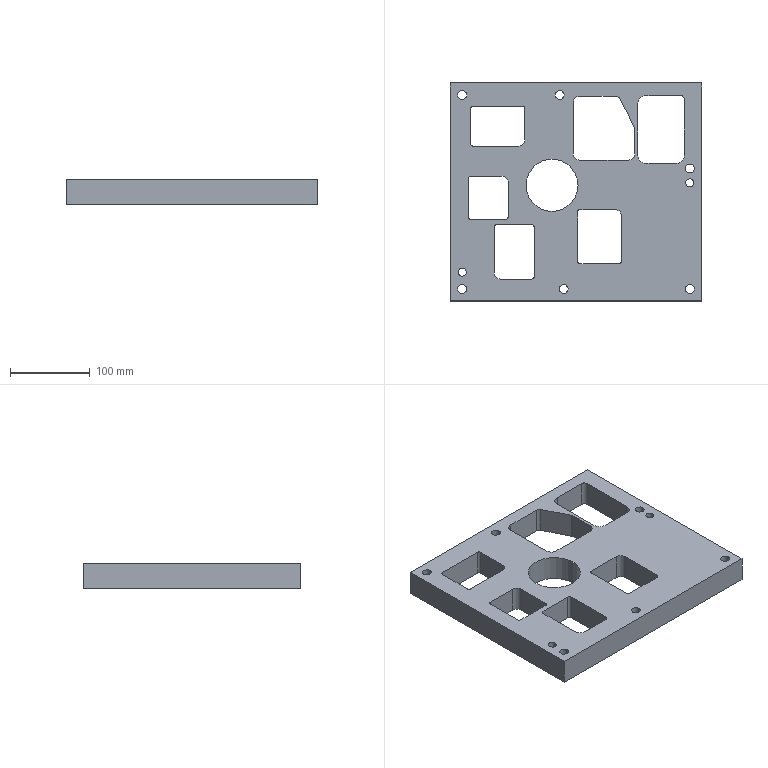Part | STEP file | lll_id3554_x_t | 1 solid | 81 faces | box 315 x 273 x 32 mm | volume 1846250 mm3 | cylinder 42 | plane 37 | cone 2 | commonest cylinder face diameters 6 x12 16 x7 11 x6 17 x6 10 x5 20 x3